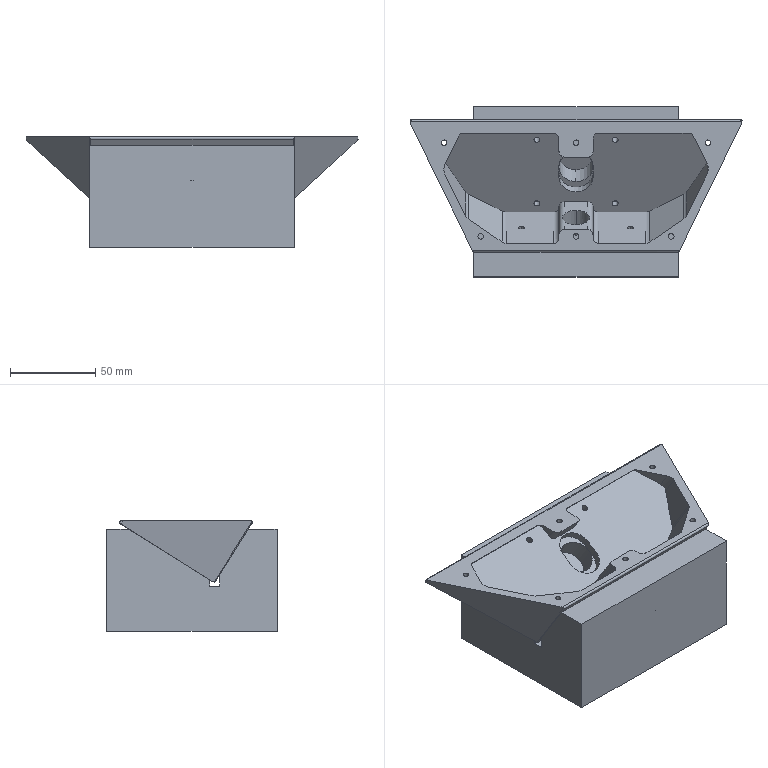CAM job | Mastercam | 3-axis milling, drilling | part box 195.124 x 100 x 65 mm
Tools:
tool_number,name,type,diameter_mm,corner_radius_mm,flutes,flute_length_mm,overall_length_mm,shoulder_length_mm,holder_diameter_mm,length_offset,diameter_offset,default_rpm,default_feed_mm_min,default_plunge_mm_min,coolant
1,16 Roughing cutter,end mill,16,0,4,25,50,25,50,1,1,4000,800,2000,COOL_OFF
1,50 Facing,end mill,50,0,4,5,50,18,50,1,1,5000,700,2000,COOL_OFF
2,50 Facing,end mill,50,0,4,5,50,18,50,2,2,5000,700,2000,COOL_OFF
2,16 Finish cutter,end mill,16,0,4,25,50,25,50,2,2,4000,800,2000,COOL_OFF
3,12 Roughing cutter,end mill,12,0,4,25,50,25,50,3,3,6500,2000,2000,COOL_OFF
3,6 Spot Drill,drill,6,0,2,25,30,30,50,3,3,1000,120,600,COOL_OFF
4,3.3 Drill,drill,3.3,0,2,25,50,40,50,4,4,1818,218.16,600,COOL_OFF
5,M4 x 0.7 RH Tap,drill,4,0,2,20,52,20,50,5,5,1500,1050,600,COOL_OFF
5,3.2 Drill,drill,3.2,0,2,25,50,40,50,5,5,1875,225,600,COOL_OFF
6,12 Flat End Mill Rough,end mill,12,0,4,25,25,25,50,6,6,833,99.96,600,COOL_OFF
6,2.5 Flat End Mill,end mill,2.5,0,4,20,20,20,50,6,6,4000,480,600,COOL_OFF
7,6 Carbide Chamfer Mill,chamfer mill,6,0,4,25,25,25,50,7,7,4167,500.04,600,COOL_OFF
7,3.15 Thread Mill,thread mill,3.15,0,4,2.1,20,20,50,7,7,1905,228.6,600,COOL_OFF
7,12 Flat End Mill Finish,end mill,12,0,4,25,25,25,50,7,7,833,99.96,600,COOL_OFF
8,16 Roughing cutter,end mill,16,0,4,25,50,25,50,8,8,5500,2000,2000,COOL_OFF
8,16 Bull Nose Mill,bull end mill,16,0.8,4,25,50,25,50,8,8,750,90,600,COOL_OFF
9,6 Flat End Mill,end mill,6,0,4,20,20,20,27.508,9,9,1667,200.04,600,COOL_OFF
10,8 Ball Mill,ball end mill,8,4,4,30,30,30,50,10,10,1500,180,600,COOL_OFF
11,3.5 Drill,drill,3.5,0,2,25,50,40,50,11,11,1714,205.68,600,COOL_OFF
11,10.3 Drill,drill,10.3,0,2,25,50,40,31.877,11,11,583,69.96,600,COOL_OFF
12,10 Flat End Mill,end mill,10,0,4,40,40,40,50,12,12,1000,120,600,COOL_OFF
12,6 Chamfer Mill,chamfer mill,6,0,4,25,25,25,50,12,12,4167,500.04,600,COOL_OFF
12,M12 x 1.75 RH Tap,drill,12,0,2,38,82,38,50,12,12,500,875.0,600,COOL_OFF
13,10 Flat End Mill Finish,end mill,10,0,4,30,30,30,31.877,13,13,1000,120,600,COOL_OFF
14,4.5 Drill,drill,4.5,0,2,25,50,40,50,14,14,1333,159.96,600,COOL_OFF
15,8 Flat End Mill Rough,end mill,8,0,4,20,20,20,50,15,15,1250,150,600,COOL_OFF
16,9 Drill,drill,9,0,2,25,50,40,50,16,16,667,80.04,600,COOL_OFF
17,8 Flat End Mill Finish,end mill,8,0,4,20,20,20,50,17,17,1250,150,600,COOL_OFF
18,14 Flat End Mill,end mill,14,0,4,25,25,25,50,18,18,714,85.68,600,COOL_OFF
Operations:
seq,operation,operation_type,tool_number,tool_name,tool_diameter_mm,spindle_rpm,feed_mm_min,plunge_mm_min,retract_mm_min,cycle_time_s,wcs,posted,nc_file
1,Contour (2D) - [WCS: Top] - [Tplane: Top],Contour,1,50 Facing,50,2300,3000,2000,5000,10.844,Top,yes,1.nc
2,Contour (2D) - [WCS: Top] - [Tplane: Top],Contour,1,50 Facing,50,2300,3000,2000,5000,11.313,Top,yes,1.nc
3,Contour (2D) - [WCS: Top] - [Tplane: Top],Contour,2,16 Finish cutter,16,4000,800,2000,5000,36.832,Top,yes,1.nc
4,Contour (2D) - [WCS: Top] - [Tplane: Top],Contour,2,16 Finish cutter,16,4000,800,2000,5000,38.593,Top,yes,1.nc
5,Drill/Counterbore - [WCS: Top] - [Tplane: Top],Drill,3,6 Spot Drill,6,2000,100,600,1200,13.709,Top,yes,1.nc
6,Peck Drill - [WCS: Top] - [Tplane: Top],Drill,4,3.3 Drill,3.3,1200,100,600,1200,12,Top,yes,1.nc
7,Peck Drill - [WCS: Top] - [Tplane: Top],Drill,4,3.3 Drill,3.3,1200,100,600,1200,11.395,Top,yes,1.nc
8,Drill/Counterbore - [WCS: Top] - [Tplane: Top],Drill,5,3.2 Drill,3.2,1200,100,600,1200,11.827,Top,yes,1.nc
9,Drill/Counterbore - [WCS: Top] - [Tplane: Top],Drill,5,3.2 Drill,3.2,1200,100,600,1200,11.827,Top,yes,1.nc
10,Circle Mill - [WCS: Top] - [Tplane: Top],CircleMill,6,2.5 Flat End Mill,2.5,3500,100,600,1200,11.987,Top,yes,1.nc
11,Thread Mill - [WCS: Top] - [Tplane: Top],ThreadMill,7,12 Flat End Mill Finish,12,3000,200,600,1200,147.861,Top,yes,1.nc
12,Contour (Ramp) - [WCS: Top] - [Tplane: Fx1-1],Contour,8,16 Bull Nose Mill,16,5500,2000,2000,5000,465.924,Top,yes,3.nc
13,Surface Rough Pocket - [WCS: Top] - [Tplane: Fx1-1],MultiSurfaceRoughPocket,8,16 Bull Nose Mill,16,5500,2000,2000,5000,491.104,Top,yes,3.nc
14,Contour (2D) - [WCS: Top] - [Tplane: Fx1-1],Contour,2,16 Finish cutter,16,4000,800,2000,5000,79.56,Top,yes,3.nc
15,Contour (Ramp) - [WCS: Top] - [Tplane: Fx1-1],Contour,9,6 Flat End Mill,6,5000,1500,2000,1200,74.171,Top,yes,3.nc
16,Stock model - [WCS: Fx1-1] - [Tplane: Fx1-1] - 2,139,,,,0,0,0,0,0,Fx1-1,yes,1.nc|2.nc|3.nc
17,Surface Finish Flowline - [WCS: Top] - [Tplane: Fx1-1],MultiSurfaceFinishFlowline,10,8 Ball Mill,8,5500,3500,2000,1200,1301.724,Top,yes,3.nc
18,Drill/Counterbore - [WCS: Top] - [Tplane: Fx1-2],Drill,3,6 Spot Drill,6,3000,300,600,1200,1.011,Top,yes,3.nc
19,Peck Drill - [WCS: Top] - [Tplane: Fx1-2],Drill,11,10.3 Drill,10.3,3000,300,600,1200,8.918,Top,yes,3.nc
20,Tap - [WCS: Top] - [Tplane: Fx1-2],Drill,12,M12 x 1.75 RH Tap,12,200,350,600,1200,11.685,Top,yes,3.nc
21,Contour (Ramp) - [WCS: Top] - [Tplane: Fx1-3],Contour,13,10 Flat End Mill Finish,10,4500,1500,2000,1200,33.899,Top,yes,3.nc
22,Contour (2D) - [WCS: Top] - [Tplane: Fx1-3],Contour,13,10 Flat End Mill Finish,10,4500,600,2000,1200,0,Top,no,
23,2D High Speed (2D Dynamic Mill) - [WCS: Top] - [Tplane: Fixture 2-1],HighSpeed2D,8,16 Bull Nose Mill,16,5000,4000,2000,1200,447.645,Top,yes,3.nc
24,Contour (2D) - [WCS: Top] - [Tplane: Fixture 2-1],Contour,2,16 Finish cutter,16,4000,800,2000,5000,98.385,Top,yes,3.nc
25,Drill/Counterbore - [WCS: Top] - [Tplane: Fixture 2-1],Drill,3,6 Spot Drill,6,3000,300,600,1200,6.509,Top,yes,3.nc
26,Peck Drill - [WCS: Top] - [Tplane: Fixture 2-1],Drill,14,4.5 Drill,4.5,3000,300,600,1200,37.338,Top,yes,3.nc
27,Drill/Counterbore - [WCS: Top] - [Tplane: Fixture 2-1],Drill,15,8 Flat End Mill Rough,8,2000,100,600,1200,28.493,Top,yes,3.nc
28,Peck Drill - [WCS: Top] - [Tplane: Fixture 2-1],Drill,16,9 Drill,9,3000,300,600,1200,24.851,Top,yes,3.nc
29,Contour (Ramp) - [WCS: Top] - [Tplane: Fixture 2-1],Contour,15,8 Flat End Mill Rough,8,4500,800,2000,1200,20.179,Top,yes,3.nc
30,Contour (2D) - [WCS: Top] - [Tplane: Fixture 2-1],Contour,17,8 Flat End Mill Finish,8,4500,400,2000,1200,10.699,Top,yes,3.nc
31,Contour (2D chamfer) - [WCS: Top] - [Tplane: Fixture 2-1],Contour,3,6 Spot Drill,6,4000,600,2000,1200,85.509,Top,yes,3.nc
32,Drill/Counterbore - [WCS: Top] - [Tplane: Fixture 2-2],Drill,18,14 Flat End Mill,14,1000,100,600,1200,32.294,Top,yes,3.nc
33,2D High Speed (2D Dynamic Mill) - [WCS: Top] - [Tplane: Fixture 2-2],HighSpeed2D,6,2.5 Flat End Mill,2.5,6500,4000,2000,1200,835.934,Top,yes,3.nc
34,2D High Speed (2D Dynamic Mill) - [WCS: Top] - [Tplane: Fixture 2-2],HighSpeed2D,6,2.5 Flat End Mill,2.5,6500,4000,2000,1200,4.279,Top,yes,3.nc
35,Contour (Ramp) - [WCS: Top] - [Tplane: Fixture 2-2],Contour,6,2.5 Flat End Mill,2.5,7000,1500,2000,5000,11.867,Top,yes,3.nc
36,Pocket (Standard) - [WCS: Top] - [Tplane: Fixture 2-2],Pocket,7,12 Flat End Mill Finish,12,6500,1000,2000,5000,183.786,Top,yes,3.nc
37,Contour (2D) - [WCS: Top] - [Tplane: Fixture 2-2],Contour,7,12 Flat End Mill Finish,12,6000,500,500,5000,27.026,Top,yes,3.nc
38,Contour (2D) - [WCS: Top] - [Tplane: Fixture 2-2],Contour,7,12 Flat End Mill Finish,12,7000,600,2000,5000,6.892,Top,yes,3.nc
39,Contour (2D chamfer) - [WCS: Top] - [Tplane: Fixture 2-2],Contour,3,6 Spot Drill,6,4000,600,2000,1200,77.105,Top,yes,3.nc
40,Contour (2D chamfer) - [WCS: Top] - [Tplane: Fixture 2-2],Contour,3,6 Spot Drill,6,4000,600,2000,1200,4.959,Top,yes,3.nc
41,Facing - [WCS: Top] - [Tplane: 1],Facing,1,50 Facing,50,2300,3500,2000,5000,160.94,Top,yes,1.nc
42,Facing - [WCS: Top] - [Tplane: 2],Facing,1,50 Facing,50,2300,3500,2000,5000,83.438,Top,yes,1.nc
43,Facing - [WCS: Top] - [Tplane: 3],Facing,1,50 Facing,50,2300,3500,2000,5000,48.002,Top,yes,1.nc
44,Facing - [WCS: Top] - [Tplane: 4],Facing,1,50 Facing,50,2300,3500,2000,5000,43.512,Top,yes,1.nc
45,Contour (Ramp) - [WCS: Top] - [Tplane: 5],Contour,1,50 Facing,50,2300,3500,2000,5000,7.65,Top,yes,1.nc
46,Contour (Ramp) - [WCS: Top] - [Tplane: 6],Contour,1,50 Facing,50,2300,3500,2000,5000,7.65,Top,yes,1.nc
47,Facing - [WCS: Top] - [Tplane: 1],Facing,2,16 Finish cutter,16,4500,600,2000,5000,116.45,Top,yes,1.nc
48,Facing - [WCS: Top] - [Tplane: 2],Facing,2,16 Finish cutter,16,4500,600,2000,5000,60.413,Top,yes,1.nc
49,Facing - [WCS: Top] - [Tplane: 3],Facing,2,16 Finish cutter,16,4500,600,2000,5000,34.203,Top,yes,1.nc
50,Facing - [WCS: Top] - [Tplane: 4],Facing,2,16 Finish cutter,16,4500,600,2000,5000,30.832,Top,yes,1.nc
51,Contour (2D) - [WCS: Top] - [Tplane: 5],Contour,2,16 Finish cutter,16,4500,600,2000,5000,5.565,Top,yes,1.nc
52,Contour (2D) - [WCS: Top] - [Tplane: 6],Contour,2,16 Finish cutter,16,4500,600,2000,5000,5.565,Top,yes,1.nc
53,Drill/Counterbore - [WCS: Top] - [Tplane: 1],Drill,3,6 Spot Drill,6,2000,100,600,1200,7.589,Top,yes,1.nc
54,Drill/Counterbore - [WCS: Top] - [Tplane: 2],Drill,3,6 Spot Drill,6,2000,100,600,1200,4.097,Top,yes,1.nc
55,Drill/Counterbore - [WCS: Top] - [Tplane: 2],Drill,4,3.3 Drill,3.3,1200,100,600,1200,11.345,Top,yes,1.nc
56,Tap - [WCS: Top] - [Tplane: 2],Drill,5,3.2 Drill,3.2,300,210.0,600,1200,27.093,Top,yes,1.nc
57,Drill/Counterbore - [WCS: Top] - [Tplane: 1],Drill,11,10.3 Drill,10.3,1200,100,600,1200,22.691,Top,yes,1.nc
58,Contour (2D chamfer) - [WCS: Top] - [Tplane: 1],Contour,7,12 Flat End Mill Finish,12,3500,800,2000,1200,21.095,Top,yes,1.nc
59,Drill/Counterbore - [WCS: Top] - [Tplane: Top],Drill,3,6 Spot Drill,6,3000,300,600,1200,1.642,Top,yes,2.nc